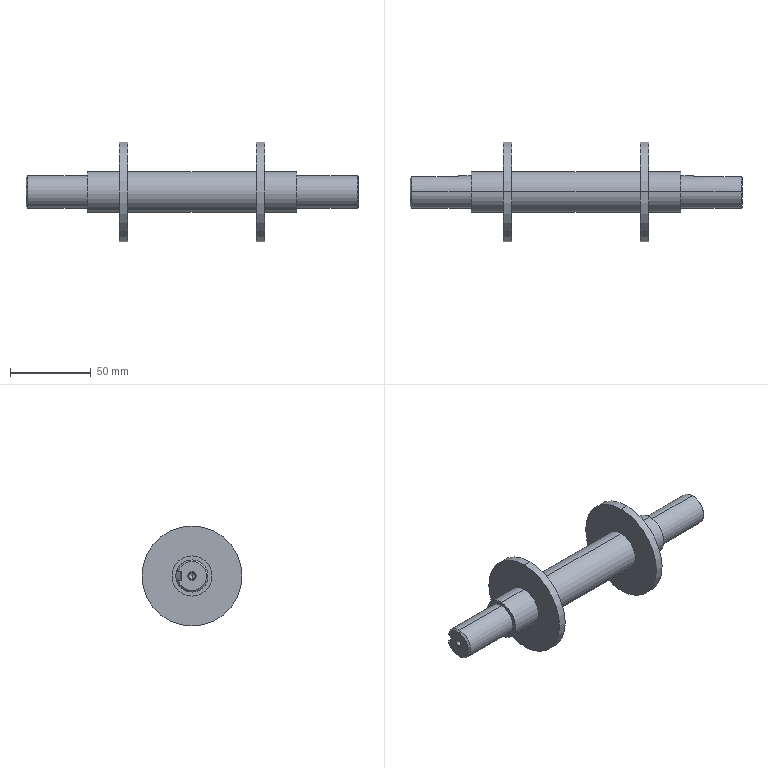Part | SolidWorks | features BaseBody 1 | 1 solid | 48 faces | box 206 x 62 x 62 mm | volume 111425 mm3 | cylinder 18 | cone 14 | plane 14 | spline 2 | commonest cylinder face diameters 25 x6 4.2 x4 20 x4 62 x4
STEP:
#1=CARTESIAN_POINT('',(102.5,0.,2.1));
#2=VERTEX_POINT('',#1);
#3=CARTESIAN_POINT('',(102.5,0.,-2.1));
#4=VERTEX_POINT('',#3);
#5=CARTESIAN_POINT('',(102.5,0.,0.));
#6=DIRECTION('',(1.,0.,0.));
#7=DIRECTION('',(0.,0.,-1.));
#8=AXIS2_PLACEMENT_3D('',#5,#6,#7);
#9=CIRCLE('',#8,2.1);
#10=EDGE_CURVE('',#2,#4,#9,.T.);
#11=ORIENTED_EDGE('',*,*,#10,.F.);
#12=CARTESIAN_POINT('',(103.,0.,2.6));
#13=VERTEX_POINT('',#12);
#14=CARTESIAN_POINT('',(102.5,0.,2.1));
#15=DIRECTION('',(0.7071,0.,0.7071));
#16=VECTOR('',#15,1000.);
#17=LINE('',#14,#16);
#18=EDGE_CURVE('',#2,#13,#17,.T.);
#19=ORIENTED_EDGE('',*,*,#18,.T.);
#20=CARTESIAN_POINT('',(103.,0.,-2.6));
#21=VERTEX_POINT('',#20);
#22=CARTESIAN_POINT('',(103.,0.,0.));
#23=DIRECTION('',(-1.,0.,0.));
#24=DIRECTION('',(0.,0.,-1.));
#25=AXIS2_PLACEMENT_3D('',#22,#23,#24);
#26=CIRCLE('',#25,2.6);
#27=EDGE_CURVE('',#21,#13,#26,.T.);
#28=ORIENTED_EDGE('',*,*,#27,.F.);
#29=CARTESIAN_POINT('',(102.5,0.,-2.1));
#30=DIRECTION('',(0.7071,0.,-0.7071));
#31=VECTOR('',#30,1000.);
#32=LINE('',#29,#31);
#33=EDGE_CURVE('',#4,#21,#32,.T.);
#34=ORIENTED_EDGE('',*,*,#33,.F.);
#35=EDGE_LOOP('',(#11,#19,#28,#34));
#36=FACE_OUTER_BOUND('',#35,.T.);
#37=CARTESIAN_POINT('',(102.5,0.,0.));
#38=DIRECTION('',(1.,0.,0.));
#39=DIRECTION('',(0.,0.,-1.));
#40=AXIS2_PLACEMENT_3D('',#37,#38,#39);
#41=CONICAL_SURFACE('',#40,2.1,0.7854);
#42=ADVANCED_FACE('',(#36),#41,.F.);
#43=CARTESIAN_POINT('',(-102.5,0.,-2.1));
#44=VERTEX_POINT('',#43);
#45=CARTESIAN_POINT('',(-102.5,0.,2.1));
#46=VERTEX_POINT('',#45);
#47=CARTESIAN_POINT('',(-102.5,0.,0.));
#48=DIRECTION('',(-1.,0.,0.));
#49=DIRECTION('',(0.,0.,1.));
#50=AXIS2_PLACEMENT_3D('',#47,#48,#49);
#51=CIRCLE('',#50,2.1);
#52=EDGE_CURVE('',#44,#46,#51,.T.);
#53=ORIENTED_EDGE('',*,*,#52,.F.);
#54=CARTESIAN_POINT('',(-103.,0.,-2.6));
#55=VERTEX_POINT('',#54);
#56=CARTESIAN_POINT('',(-102.5,0.,-2.1));
#57=DIRECTION('',(-0.7071,0.,-0.7071));
#58=VECTOR('',#57,1000.);
#59=LINE('',#56,#58);
#60=EDGE_CURVE('',#44,#55,#59,.T.);
#61=ORIENTED_EDGE('',*,*,#60,.T.);
#62=CARTESIAN_POINT('',(-103.,0.,2.6));
#63=VERTEX_POINT('',#62);
#64=CARTESIAN_POINT('',(-103.,0.,0.));
#65=DIRECTION('',(1.,0.,0.));
#66=DIRECTION('',(0.,0.,1.));
#67=AXIS2_PLACEMENT_3D('',#64,#65,#66);
#68=CIRCLE('',#67,2.6);
#69=EDGE_CURVE('',#63,#55,#68,.T.);
#70=ORIENTED_EDGE('',*,*,#69,.F.);
#71=CARTESIAN_POINT('',(-102.5,0.,2.1));
#72=DIRECTION('',(-0.7071,0.,0.7071));
#73=VECTOR('',#72,1000.);
#74=LINE('',#71,#73);
#75=EDGE_CURVE('',#46,#63,#74,.T.);
#76=ORIENTED_EDGE('',*,*,#75,.F.);
#77=EDGE_LOOP('',(#53,#61,#70,#76));
#78=FACE_OUTER_BOUND('',#77,.T.);
#79=CARTESIAN_POINT('',(-102.5,0.,0.));
#80=DIRECTION('',(-1.,0.,0.));
#81=DIRECTION('',(0.,0.,1.));
#82=AXIS2_PLACEMENT_3D('',#79,#80,#81);
#83=CONICAL_SURFACE('',#82,2.1,0.7854);
#84=ADVANCED_FACE('',(#78),#83,.F.);
#85=CARTESIAN_POINT('',(90.6,0.,2.1));
#86=VERTEX_POINT('',#85);
#87=CARTESIAN_POINT('',(90.6,0.,-2.1));
#88=VERTEX_POINT('',#87);
#89=CARTESIAN_POINT('',(90.6,0.,0.));
#90=DIRECTION('',(1.,0.,0.));
#91=DIRECTION('',(0.,0.,-1.));
#92=AXIS2_PLACEMENT_3D('',#89,#90,#91);
#93=CIRCLE('',#92,2.1);
#94=EDGE_CURVE('',#86,#88,#93,.T.);
#95=ORIENTED_EDGE('',*,*,#94,.F.);
#96=CARTESIAN_POINT('',(103.,0.,2.1));
#97=DIRECTION('',(1.,0.,0.));
#98=VECTOR('',#97,1000.);
#99=LINE('',#96,#98);
#100=EDGE_CURVE('',#86,#2,#99,.T.);
#101=ORIENTED_EDGE('',*,*,#100,.T.);
#102=ORIENTED_EDGE('',*,*,#10,.T.);
#103=CARTESIAN_POINT('',(103.,0.,-2.1));
#104=DIRECTION('',(1.,0.,0.));
#105=VECTOR('',#104,1000.);
#106=LINE('',#103,#105);
#107=EDGE_CURVE('',#88,#4,#106,.T.);
#108=ORIENTED_EDGE('',*,*,#107,.F.);
#109=EDGE_LOOP('',(#95,#101,#102,#108));
#110=FACE_OUTER_BOUND('',#109,.T.);
#111=CARTESIAN_POINT('',(103.,0.,0.));
#112=DIRECTION('',(1.,0.,0.));
#113=DIRECTION('',(0.,0.,-1.));
#114=AXIS2_PLACEMENT_3D('',#111,#112,#113);
#115=CYLINDRICAL_SURFACE('',#114,2.1);
#116=ADVANCED_FACE('',(#110),#115,.F.);
#117=CARTESIAN_POINT('',(89.338,0.,0.));
#118=VERTEX_POINT('',#117);
#119=CARTESIAN_POINT('',(90.6,0.,-2.1));
#120=DIRECTION('',(0.515,0.,-0.8572));
#121=VECTOR('',#120,1000.);
#122=LINE('',#119,#121);
#123=EDGE_CURVE('',#118,#88,#122,.T.);
#124=ORIENTED_EDGE('',*,*,#123,.F.);
#125=CARTESIAN_POINT('',(90.6,0.,2.1));
#126=DIRECTION('',(0.515,0.,0.8572));
#127=VECTOR('',#126,1000.);
#128=LINE('',#125,#127);
#129=EDGE_CURVE('',#118,#86,#128,.T.);
#130=ORIENTED_EDGE('',*,*,#129,.T.);
#131=ORIENTED_EDGE('',*,*,#94,.T.);
#132=EDGE_LOOP('',(#124,#130,#131));
#133=FACE_OUTER_BOUND('',#132,.T.);
#134=CARTESIAN_POINT('',(90.6,0.,0.));
#135=DIRECTION('',(1.,0.,0.));
#136=DIRECTION('',(0.,0.,-1.));
#137=AXIS2_PLACEMENT_3D('',#134,#135,#136);
#138=CONICAL_SURFACE('',#137,2.1,1.03);
#139=ADVANCED_FACE('',(#133),#138,.F.);
#140=CARTESIAN_POINT('',(-90.6,0.,-2.1));
#141=VERTEX_POINT('',#140);
#142=CARTESIAN_POINT('',(-90.6,0.,2.1));
#143=VERTEX_POINT('',#142);
#144=CARTESIAN_POINT('',(-90.6,0.,0.));
#145=DIRECTION('',(-1.,0.,0.));
#146=DIRECTION('',(0.,0.,1.));
#147=AXIS2_PLACEMENT_3D('',#144,#145,#146);
#148=CIRCLE('',#147,2.1);
#149=EDGE_CURVE('',#141,#143,#148,.T.);
#150=ORIENTED_EDGE('',*,*,#149,.F.);
#151=CARTESIAN_POINT('',(-103.,0.,-2.1));
#152=DIRECTION('',(-1.,0.,0.));
#153=VECTOR('',#152,1000.);
#154=LINE('',#151,#153);
#155=EDGE_CURVE('',#141,#44,#154,.T.);
#156=ORIENTED_EDGE('',*,*,#155,.T.);
#157=ORIENTED_EDGE('',*,*,#52,.T.);
#158=CARTESIAN_POINT('',(-103.,0.,2.1));
#159=DIRECTION('',(-1.,0.,0.));
#160=VECTOR('',#159,1000.);
#161=LINE('',#158,#160);
#162=EDGE_CURVE('',#143,#46,#161,.T.);
#163=ORIENTED_EDGE('',*,*,#162,.F.);
#164=EDGE_LOOP('',(#150,#156,#157,#163));
#165=FACE_OUTER_BOUND('',#164,.T.);
#166=CARTESIAN_POINT('',(-103.,0.,0.));
#167=DIRECTION('',(-1.,0.,0.));
#168=DIRECTION('',(0.,0.,1.));
#169=AXIS2_PLACEMENT_3D('',#166,#167,#168);
#170=CYLINDRICAL_SURFACE('',#169,2.1);
#171=ADVANCED_FACE('',(#165),#170,.F.);
#172=CARTESIAN_POINT('',(-89.338,0.,0.));
#173=VERTEX_POINT('',#172);
#174=CARTESIAN_POINT('',(-90.6,0.,2.1));
#175=DIRECTION('',(-0.515,0.,0.8572));
#176=VECTOR('',#175,1000.);
#177=LINE('',#174,#176);
#178=EDGE_CURVE('',#173,#143,#177,.T.);
#179=ORIENTED_EDGE('',*,*,#178,.F.);
#180=CARTESIAN_POINT('',(-90.6,0.,-2.1));
#181=DIRECTION('',(-0.515,0.,-0.8572));
#182=VECTOR('',#181,1000.);
#183=LINE('',#180,#182);
#184=EDGE_CURVE('',#173,#141,#183,.T.);
#185=ORIENTED_EDGE('',*,*,#184,.T.);
#186=ORIENTED_EDGE('',*,*,#149,.T.);
#187=EDGE_LOOP('',(#179,#185,#186));
#188=FACE_OUTER_BOUND('',#187,.T.);
#189=CARTESIAN_POINT('',(-90.6,0.,0.));
#190=DIRECTION('',(-1.,0.,0.));
#191=DIRECTION('',(0.,0.,1.));
#192=AXIS2_PLACEMENT_3D('',#189,#190,#191);
#193=CONICAL_SURFACE('',#192,2.1,1.03);
#194=ADVANCED_FACE('',(#188),#193,.F.);
#195=CARTESIAN_POINT('',(-103.,0.,9.));
#196=VERTEX_POINT('',#195);
#197=CARTESIAN_POINT('',(-103.,8.485,3.));
#198=VERTEX_POINT('',#197);
#199=CARTESIAN_POINT('',(-103.,0.,0.));
#200=DIRECTION('',(-1.,0.,0.));
#201=DIRECTION('',(0.,0.,1.));
#202=AXIS2_PLACEMENT_3D('',#199,#200,#201);
#203=CIRCLE('',#202,9.);
#204=EDGE_CURVE('',#196,#198,#203,.T.);
#205=ORIENTED_EDGE('',*,*,#204,.F.);
#206=CARTESIAN_POINT('',(-102.,0.,10.));
#207=VERTEX_POINT('',#206);
#208=CARTESIAN_POINT('',(-103.,0.,9.));
#209=DIRECTION('',(0.7071,0.,0.7071));
#210=VECTOR('',#209,1000.);
#211=LINE('',#208,#210);
#212=EDGE_CURVE('',#196,#207,#211,.T.);
#213=ORIENTED_EDGE('',*,*,#212,.T.);
#214=CARTESIAN_POINT('',(-102.,9.539,3.));
#215=VERTEX_POINT('',#214);
#216=CARTESIAN_POINT('',(-102.,0.,0.));
#217=DIRECTION('',(1.,0.,0.));
#218=DIRECTION('',(0.,0.,1.));
#219=AXIS2_PLACEMENT_3D('',#216,#217,#218);
#220=CIRCLE('',#219,10.);
#221=EDGE_CURVE('',#215,#207,#220,.T.);
#222=ORIENTED_EDGE('',*,*,#221,.F.);
#223=CARTESIAN_POINT('',(-103.,8.485,3.));
#224=CARTESIAN_POINT('',(-102.668,8.838,3.));
#225=CARTESIAN_POINT('',(-102.334,9.189,3.));
#226=CARTESIAN_POINT('',(-102.,9.539,3.));
#227=B_SPLINE_CURVE_WITH_KNOTS('',3,(#223,#224,#225,#226),.UNSPECIFIED.,.F.,.F.,(4,4),(0.006491,0.007944),.UNSPECIFIED.);
#228=EDGE_CURVE('',#198,#215,#227,.T.);
#229=ORIENTED_EDGE('',*,*,#228,.F.);
#230=EDGE_LOOP('',(#205,#213,#222,#229));
#231=FACE_OUTER_BOUND('',#230,.T.);
#232=CARTESIAN_POINT('',(-103.,0.,0.));
#233=DIRECTION('',(1.,0.,0.));
#234=DIRECTION('',(0.,0.,-1.));
#235=AXIS2_PLACEMENT_3D('',#232,#233,#234);
#236=CONICAL_SURFACE('',#235,9.,0.7854);
#237=ADVANCED_FACE('',(#231),#236,.T.);
#238=ORIENTED_EDGE('',*,*,#212,.F.);
#239=CARTESIAN_POINT('',(-103.,0.,-9.));
#240=VERTEX_POINT('',#239);
#241=CARTESIAN_POINT('',(-103.,0.,0.));
#242=DIRECTION('',(-1.,0.,0.));
#243=DIRECTION('',(0.,0.,1.));
#244=AXIS2_PLACEMENT_3D('',#241,#242,#243);
#245=CIRCLE('',#244,9.);
#246=EDGE_CURVE('',#240,#196,#245,.T.);
#247=ORIENTED_EDGE('',*,*,#246,.F.);
#248=CARTESIAN_POINT('',(-102.,0.,-10.));
#249=VERTEX_POINT('',#248);
#250=CARTESIAN_POINT('',(-103.,0.,-9.));
#251=DIRECTION('',(0.7071,0.,-0.7071));
#252=VECTOR('',#251,1000.);
#253=LINE('',#250,#252);
#254=EDGE_CURVE('',#240,#249,#253,.T.);
#255=ORIENTED_EDGE('',*,*,#254,.T.);
#256=CARTESIAN_POINT('',(-102.,0.,0.));
#257=DIRECTION('',(1.,0.,0.));
#258=DIRECTION('',(0.,0.,1.));
#259=AXIS2_PLACEMENT_3D('',#256,#257,#258);
#260=CIRCLE('',#259,10.);
#261=EDGE_CURVE('',#207,#249,#260,.T.);
#262=ORIENTED_EDGE('',*,*,#261,.F.);
#263=EDGE_LOOP('',(#238,#247,#255,#262));
#264=FACE_OUTER_BOUND('',#263,.T.);
#265=CARTESIAN_POINT('',(-103.,0.,0.));
#266=DIRECTION('',(1.,0.,0.));
#267=DIRECTION('',(0.,0.,-1.));
#268=AXIS2_PLACEMENT_3D('',#265,#266,#267);
#269=CONICAL_SURFACE('',#268,9.,0.7854);
#270=ADVANCED_FACE('',(#264),#269,.T.);
#271=ORIENTED_EDGE('',*,*,#221,.T.);
#272=CARTESIAN_POINT('',(-65.,0.,10.));
#273=VERTEX_POINT('',#272);
#274=CARTESIAN_POINT('',(-103.,0.,10.));
#275=DIRECTION('',(1.,0.,0.));
#276=VECTOR('',#275,1000.);
#277=LINE('',#274,#276);
#278=EDGE_CURVE('',#207,#273,#277,.T.);
#279=ORIENTED_EDGE('',*,*,#278,.T.);
#280=CARTESIAN_POINT('',(-65.,0.,-10.));
#281=VERTEX_POINT('',#280);
#282=CARTESIAN_POINT('',(-65.,0.,0.));
#283=DIRECTION('',(-1.,0.,0.));
#284=DIRECTION('',(0.,0.,1.));
#285=AXIS2_PLACEMENT_3D('',#282,#283,#284);
#286=CIRCLE('',#285,10.);
#287=EDGE_CURVE('',#273,#281,#286,.T.);
#288=ORIENTED_EDGE('',*,*,#287,.T.);
#289=CARTESIAN_POINT('',(-103.,0.,-10.));
#290=DIRECTION('',(1.,0.,0.));
#291=VECTOR('',#290,1000.);
#292=LINE('',#289,#291);
#293=EDGE_CURVE('',#249,#281,#292,.T.);
#294=ORIENTED_EDGE('',*,*,#293,.F.);
#295=CARTESIAN_POINT('',(-102.,9.539,-3.));
#296=VERTEX_POINT('',#295);
#297=CARTESIAN_POINT('',(-102.,0.,0.));
#298=DIRECTION('',(1.,0.,0.));
#299=DIRECTION('',(0.,0.,1.));
#300=AXIS2_PLACEMENT_3D('',#297,#298,#299);
#301=CIRCLE('',#300,10.);
#302=EDGE_CURVE('',#249,#296,#301,.T.);
#303=ORIENTED_EDGE('',*,*,#302,.T.);
#304=CARTESIAN_POINT('',(-73.,9.539,-3.));
#305=VERTEX_POINT('',#304);
#306=CARTESIAN_POINT('',(-103.,9.539,-3.));
#307=DIRECTION('',(1.,0.,0.));
#308=VECTOR('',#307,1000.);
#309=LINE('',#306,#308);
#310=EDGE_CURVE('',#296,#305,#309,.T.);
#311=ORIENTED_EDGE('',*,*,#310,.T.);
#312=CARTESIAN_POINT('',(-73.,9.539,3.));
#313=VERTEX_POINT('',#312);
#314=CARTESIAN_POINT('',(-73.,9.539,-3.));
#315=CARTESIAN_POINT('',(-73.,9.692,-2.514));
#316=CARTESIAN_POINT('',(-73.,9.807,-2.019));
#317=CARTESIAN_POINT('',(-73.,9.962,-1.011));
#318=CARTESIAN_POINT('',(-73.,10.,-0.5036));
#319=CARTESIAN_POINT('',(-73.,10.,0.5143));
#320=CARTESIAN_POINT('',(-73.,9.96,1.022));
#321=CARTESIAN_POINT('',(-73.,9.807,2.021));
#322=CARTESIAN_POINT('',(-73.,9.692,2.514));
#323=CARTESIAN_POINT('',(-73.,9.539,3.));
#324=B_SPLINE_CURVE_WITH_KNOTS('',3,(#314,#315,#316,#317,#318,#319,#320,#321,#322,#323),.UNSPECIFIED.,.F.,.F.,(4,2,2,2,4),(0.,0.001525,0.003049,0.004574,0.006098),.UNSPECIFIED.);
#325=EDGE_CURVE('',#305,#313,#324,.T.);
#326=ORIENTED_EDGE('',*,*,#325,.T.);
#327=CARTESIAN_POINT('',(-103.,9.539,3.));
#328=DIRECTION('',(-1.,0.,0.));
#329=VECTOR('',#328,1000.);
#330=LINE('',#327,#329);
#331=EDGE_CURVE('',#313,#215,#330,.T.);
#332=ORIENTED_EDGE('',*,*,#331,.T.);
#333=EDGE_LOOP('',(#271,#279,#288,#294,#303,#311,#326,#332));
#334=FACE_OUTER_BOUND('',#333,.T.);
#335=CARTESIAN_POINT('',(-103.,0.,0.));
#336=DIRECTION('',(1.,0.,0.));
#337=DIRECTION('',(0.,0.,-1.));
#338=AXIS2_PLACEMENT_3D('',#335,#336,#337);
#339=CYLINDRICAL_SURFACE('',#338,10.);
#340=ADVANCED_FACE('',(#334),#339,.T.);
#341=CARTESIAN_POINT('',(65.,0.,12.5));
#342=VERTEX_POINT('',#341);
#343=CARTESIAN_POINT('',(65.,0.,-12.5));
#344=VERTEX_POINT('',#343);
#345=CARTESIAN_POINT('',(65.,0.,0.));
#346=DIRECTION('',(-1.,0.,0.));
#347=DIRECTION('',(0.,0.,1.));
#348=AXIS2_PLACEMENT_3D('',#345,#346,#347);
#349=CIRCLE('',#348,12.5);
#350=EDGE_CURVE('',#342,#344,#349,.T.);
#351=ORIENTED_EDGE('',*,*,#350,.T.);
#352=CARTESIAN_POINT('',(45.,0.,-12.5));
#353=VERTEX_POINT('',#352);
#354=CARTESIAN_POINT('',(-45.,0.,-12.5));
#355=DIRECTION('',(-1.,0.,0.));
#356=VECTOR('',#355,1000.);
#357=LINE('',#354,#356);
#358=EDGE_CURVE('',#344,#353,#357,.T.);
#359=ORIENTED_EDGE('',*,*,#358,.T.);
#360=CARTESIAN_POINT('',(45.,0.,12.5));
#361=VERTEX_POINT('',#360);
#362=CARTESIAN_POINT('',(45.,0.,0.));
#363=DIRECTION('',(-1.,0.,0.));
#364=DIRECTION('',(0.,0.,1.));
#365=AXIS2_PLACEMENT_3D('',#362,#363,#364);
#366=CIRCLE('',#365,12.5);
#367=EDGE_CURVE('',#361,#353,#366,.T.);
#368=ORIENTED_EDGE('',*,*,#367,.F.);
#369=CARTESIAN_POINT('',(-45.,0.,12.5));
#370=DIRECTION('',(-1.,0.,0.));
#371=VECTOR('',#370,1000.);
#372=LINE('',#369,#371);
#373=EDGE_CURVE('',#342,#361,#372,.T.);
#374=ORIENTED_EDGE('',*,*,#373,.F.);
#375=EDGE_LOOP('',(#351,#359,#368,#374));
#376=FACE_OUTER_BOUND('',#375,.T.);
#377=CARTESIAN_POINT('',(-45.,0.,0.));
#378=DIRECTION('',(-1.,0.,0.));
#379=DIRECTION('',(0.,0.,1.));
#380=AXIS2_PLACEMENT_3D('',#377,#378,#379);
#381=CYLINDRICAL_SURFACE('',#380,12.5);
#382=ADVANCED_FACE('',(#376),#381,.T.);
#383=CARTESIAN_POINT('',(45.,0.,31.));
#384=VERTEX_POINT('',#383);
#385=CARTESIAN_POINT('',(45.,0.,-31.));
#386=VERTEX_POINT('',#385);
#387=CARTESIAN_POINT('',(45.,0.,0.));
#388=DIRECTION('',(-1.,0.,0.));
#389=DIRECTION('',(0.,0.,1.));
#390=AXIS2_PLACEMENT_3D('',#387,#388,#389);
#391=CIRCLE('',#390,31.);
#392=EDGE_CURVE('',#384,#386,#391,.T.);
#393=ORIENTED_EDGE('',*,*,#392,.T.);
#394=CARTESIAN_POINT('',(40.,0.,-31.));
#395=VERTEX_POINT('',#394);
#396=CARTESIAN_POINT('',(-45.,0.,-31.));
#397=DIRECTION('',(-1.,0.,0.));
#398=VECTOR('',#397,1000.);
#399=LINE('',#396,#398);
#400=EDGE_CURVE('',#386,#395,#399,.T.);
#401=ORIENTED_EDGE('',*,*,#400,.T.);
#402=CARTESIAN_POINT('',(40.,0.,31.));
#403=VERTEX_POINT('',#402);
#404=CARTESIAN_POINT('',(40.,0.,0.));
#405=DIRECTION('',(1.,0.,0.));
#406=DIRECTION('',(0.,0.,-1.));
#407=AXIS2_PLACEMENT_3D('',#404,#405,#406);
#408=CIRCLE('',#407,31.);
#409=EDGE_CURVE('',#395,#403,#408,.T.);
#410=ORIENTED_EDGE('',*,*,#409,.T.);
#411=CARTESIAN_POINT('',(-45.,0.,31.));
#412=DIRECTION('',(-1.,0.,0.));
#413=VECTOR('',#412,1000.);
#414=LINE('',#411,#413);
#415=EDGE_CURVE('',#384,#403,#414,.T.);
#416=ORIENTED_EDGE('',*,*,#415,.F.);
#417=EDGE_LOOP('',(#393,#401,#410,#416));
#418=FACE_OUTER_BOUND('',#417,.T.);
#419=CARTESIAN_POINT('',(-45.,0.,0.));
#420=DIRECTION('',(-1.,0.,0.));
#421=DIRECTION('',(0.,0.,1.));
#422=AXIS2_PLACEMENT_3D('',#419,#420,#421);
#423=CYLINDRICAL_SURFACE('',#422,31.);
#424=ADVANCED_FACE('',(#418),#423,.T.);
#425=CARTESIAN_POINT('',(-45.,0.,12.5));
#426=VERTEX_POINT('',#425);
#427=CARTESIAN_POINT('',(-45.,0.,-12.5));
#428=VERTEX_POINT('',#427);
#429=CARTESIAN_POINT('',(-45.,0.,0.));
#430=DIRECTION('',(-1.,0.,0.));
#431=DIRECTION('',(0.,0.,-1.));
#432=AXIS2_PLACEMENT_3D('',#429,#430,#431);
#433=CIRCLE('',#432,12.5);
#434=EDGE_CURVE('',#426,#428,#433,.T.);
#435=ORIENTED_EDGE('',*,*,#434,.T.);
#436=CARTESIAN_POINT('',(-65.,0.,-12.5));
#437=VERTEX_POINT('',#436);
#438=CARTESIAN_POINT('',(-45.,0.,-12.5));
#439=DIRECTION('',(-1.,0.,0.));
#440=VECTOR('',#439,1000.);
#441=LINE('',#438,#440);
#442=EDGE_CURVE('',#428,#437,#441,.T.);
#443=ORIENTED_EDGE('',*,*,#442,.T.);
#444=CARTESIAN_POINT('',(-65.,0.,12.5));
#445=VERTEX_POINT('',#444);
#446=CARTESIAN_POINT('',(-65.,0.,0.));
#447=DIRECTION('',(-1.,0.,0.));
#448=DIRECTION('',(0.,0.,1.));
#449=AXIS2_PLACEMENT_3D('',#446,#447,#448);
#450=CIRCLE('',#449,12.5);
#451=EDGE_CURVE('',#445,#437,#450,.T.);
#452=ORIENTED_EDGE('',*,*,#451,.F.);
#453=CARTESIAN_POINT('',(-45.,0.,12.5));
#454=DIRECTION('',(-1.,0.,0.));
#455=VECTOR('',#454,1000.);
#456=LINE('',#453,#455);
#457=EDGE_CURVE('',#426,#445,#456,.T.);
#458=ORIENTED_EDGE('',*,*,#457,.F.);
#459=EDGE_LOOP('',(#435,#443,#452,#458));
#460=FACE_OUTER_BOUND('',#459,.T.);
#461=CARTESIAN_POINT('',(-45.,0.,0.));
#462=DIRECTION('',(-1.,0.,0.));
#463=DIRECTION('',(0.,0.,1.));
#464=AXIS2_PLACEMENT_3D('',#461,#462,#463);
#465=CYLINDRICAL_SURFACE('',#464,12.5);
#466=ADVANCED_FACE('',(#460),#465,.T.);
#467=CARTESIAN_POINT('',(-40.,0.,-31.));
#468=VERTEX_POINT('',#467);
#469=CARTESIAN_POINT('',(-40.,0.,31.));
#470=VERTEX_POINT('',#469);
#471=CARTESIAN_POINT('',(-40.,0.,0.));
#472=DIRECTION('',(1.,0.,0.));
#473=DIRECTION('',(0.,0.,-1.));
#474=AXIS2_PLACEMENT_3D('',#471,#472,#473);
#475=CIRCLE('',#474,31.);
#476=EDGE_CURVE('',#468,#470,#475,.T.);
#477=ORIENTED_EDGE('',*,*,#476,.F.);
#478=CARTESIAN_POINT('',(-45.,0.,-31.));
#479=VERTEX_POINT('',#478);
#480=CARTESIAN_POINT('',(-45.,0.,-31.));
#481=DIRECTION('',(-1.,0.,0.));
#482=VECTOR('',#481,1000.);
#483=LINE('',#480,#482);
#484=EDGE_CURVE('',#468,#479,#483,.T.);
#485=ORIENTED_EDGE('',*,*,#484,.T.);
#486=CARTESIAN_POINT('',(-45.,0.,31.));
#487=VERTEX_POINT('',#486);
#488=CARTESIAN_POINT('',(-45.,0.,0.));
#489=DIRECTION('',(-1.,0.,0.));
#490=DIRECTION('',(0.,0.,1.));
#491=AXIS2_PLACEMENT_3D('',#488,#489,#490);
#492=CIRCLE('',#491,31.);
#493=EDGE_CURVE('',#487,#479,#492,.T.);
#494=ORIENTED_EDGE('',*,*,#493,.F.);
#495=CARTESIAN_POINT('',(-45.,0.,31.));
#496=DIRECTION('',(-1.,0.,0.));
#497=VECTOR('',#496,1000.);
#498=LINE('',#495,#497);
#499=EDGE_CURVE('',#470,#487,#498,.T.);
#500=ORIENTED_EDGE('',*,*,#499,.F.);
#501=EDGE_LOOP('',(#477,#485,#494,#500));
#502=FACE_OUTER_BOUND('',#501,.T.);
#503=CARTESIAN_POINT('',(-45.,0.,0.));
#504=DIRECTION('',(-1.,0.,0.));
#505=DIRECTION('',(0.,0.,1.));
#506=AXIS2_PLACEMENT_3D('',#503,#504,#505);
#507=CYLINDRICAL_SURFACE('',#506,31.);
#508=ADVANCED_FACE('',(#502),#507,.T.);
#509=CARTESIAN_POINT('',(40.,0.,-12.5));
#510=VERTEX_POINT('',#509);
#511=CARTESIAN_POINT('',(40.,0.,12.5));
#512=VERTEX_POINT('',#511);
#513=CARTESIAN_POINT('',(40.,0.,0.));
#514=DIRECTION('',(1.,0.,0.));
#515=DIRECTION('',(0.,0.,-1.));
#516=AXIS2_PLACEMENT_3D('',#513,#514,#515);
#517=CIRCLE('',#516,12.5);
#518=EDGE_CURVE('',#510,#512,#517,.T.);
#519=ORIENTED_EDGE('',*,*,#518,.F.);
#520=CARTESIAN_POINT('',(-40.,0.,-12.5));
#521=VERTEX_POINT('',#520);
#522=CARTESIAN_POINT('',(-45.,0.,-12.5));
#523=DIRECTION('',(-1.,0.,0.));
#524=VECTOR('',#523,1000.);
#525=LINE('',#522,#524);
#526=EDGE_CURVE('',#510,#521,#525,.T.);
#527=ORIENTED_EDGE('',*,*,#526,.T.);
#528=CARTESIAN_POINT('',(-40.,0.,12.5));
#529=VERTEX_POINT('',#528);
#530=CARTESIAN_POINT('',(-40.,0.,0.));
#531=DIRECTION('',(1.,0.,0.));
#532=DIRECTION('',(0.,0.,-1.));
#533=AXIS2_PLACEMENT_3D('',#530,#531,#532);
#534=CIRCLE('',#533,12.5);
#535=EDGE_CURVE('',#521,#529,#534,.T.);
#536=ORIENTED_EDGE('',*,*,#535,.T.);
#537=CARTESIAN_POINT('',(-45.,0.,12.5));
#538=DIRECTION('',(-1.,0.,0.));
#539=VECTOR('',#538,1000.);
#540=LINE('',#537,#539);
#541=EDGE_CURVE('',#512,#529,#540,.T.);
#542=ORIENTED_EDGE('',*,*,#541,.F.);
#543=EDGE_LOOP('',(#519,#527,#536,#542));
#544=FACE_OUTER_BOUND('',#543,.T.);
#545=CARTESIAN_POINT('',(-45.,0.,0.));
#546=DIRECTION('',(-1.,0.,0.));
#547=DIRECTION('',(0.,0.,1.));
#548=AXIS2_PLACEMENT_3D('',#545,#546,#547);
#549=CYLINDRICAL_SURFACE('',#548,12.5);
#550=ADVANCED_FACE('',(#544),#549,.T.);
#551=CARTESIAN_POINT('',(103.,0.,-9.5));
#552=VERTEX_POINT('',#551);
#553=CARTESIAN_POINT('',(103.,9.014,-3.));
#554=VERTEX_POINT('',#553);
#555=CARTESIAN_POINT('',(103.,0.,0.));
#556=DIRECTION('',(1.,0.,0.));
#557=DIRECTION('',(0.,0.,-1.));
#558=AXIS2_PLACEMENT_3D('',#555,#556,#557);
#559=CIRCLE('',#558,9.5);
#560=EDGE_CURVE('',#552,#554,#559,.T.);
#561=ORIENTED_EDGE('',*,*,#560,.F.);
#562=CARTESIAN_POINT('',(102.5,0.,-10.));
#563=VERTEX_POINT('',#562);
#564=CARTESIAN_POINT('',(103.,0.,-9.5));
#565=DIRECTION('',(-0.7071,0.,-0.7071));
#566=VECTOR('',#565,1000.);
#567=LINE('',#564,#566);
#568=EDGE_CURVE('',#552,#563,#567,.T.);
#569=ORIENTED_EDGE('',*,*,#568,.T.);
#570=CARTESIAN_POINT('',(102.5,9.539,-3.));
#571=VERTEX_POINT('',#570);
#572=CARTESIAN_POINT('',(102.5,0.,0.));
#573=DIRECTION('',(-1.,0.,0.));
#574=DIRECTION('',(0.,0.,-1.));
#575=AXIS2_PLACEMENT_3D('',#572,#573,#574);
#576=CIRCLE('',#575,10.);
#577=EDGE_CURVE('',#571,#563,#576,.T.);
#578=ORIENTED_EDGE('',*,*,#577,.F.);
#579=CARTESIAN_POINT('',(102.5,9.539,-3.));
#580=CARTESIAN_POINT('',(102.667,9.364,-3.));
#581=CARTESIAN_POINT('',(102.834,9.189,-3.));
#582=CARTESIAN_POINT('',(103.,9.014,-3.));
#583=B_SPLINE_CURVE_WITH_KNOTS('',3,(#579,#580,#581,#582),.UNSPECIFIED.,.F.,.F.,(4,4),(0.005686,0.006411),.UNSPECIFIED.);
#584=EDGE_CURVE('',#571,#554,#583,.T.);
#585=ORIENTED_EDGE('',*,*,#584,.T.);
#586=EDGE_LOOP('',(#561,#569,#578,#585));
#587=FACE_OUTER_BOUND('',#586,.T.);
#588=CARTESIAN_POINT('',(103.,0.,0.));
#589=DIRECTION('',(-1.,0.,0.));
#590=DIRECTION('',(0.,0.,1.));
#591=AXIS2_PLACEMENT_3D('',#588,#589,#590);
#592=CONICAL_SURFACE('',#591,9.5,0.7854);
#593=ADVANCED_FACE('',(#587),#592,.T.);
#594=ORIENTED_EDGE('',*,*,#568,.F.);
#595=CARTESIAN_POINT('',(103.,0.,9.5));
#596=VERTEX_POINT('',#595);
#597=CARTESIAN_POINT('',(103.,0.,0.));
#598=DIRECTION('',(1.,0.,0.));
#599=DIRECTION('',(0.,0.,-1.));
#600=AXIS2_PLACEMENT_3D('',#597,#598,#599);
#601=CIRCLE('',#600,9.5);
#602=EDGE_CURVE('',#596,#552,#601,.T.);
#603=ORIENTED_EDGE('',*,*,#602,.F.);
#604=CARTESIAN_POINT('',(102.5,0.,10.));
#605=VERTEX_POINT('',#604);
#606=CARTESIAN_POINT('',(103.,0.,9.5));
#607=DIRECTION('',(-0.7071,0.,0.7071));
#608=VECTOR('',#607,1000.);
#609=LINE('',#606,#608);
#610=EDGE_CURVE('',#596,#605,#609,.T.);
#611=ORIENTED_EDGE('',*,*,#610,.T.);
#612=CARTESIAN_POINT('',(102.5,0.,0.));
#613=DIRECTION('',(-1.,0.,0.));
#614=DIRECTION('',(0.,0.,-1.));
#615=AXIS2_PLACEMENT_3D('',#612,#613,#614);
#616=CIRCLE('',#615,10.);
#617=EDGE_CURVE('',#563,#605,#616,.T.);
#618=ORIENTED_EDGE('',*,*,#617,.F.);
#619=EDGE_LOOP('',(#594,#603,#611,#618));
#620=FACE_OUTER_BOUND('',#619,.T.);
#621=CARTESIAN_POINT('',(103.,0.,0.));
#622=DIRECTION('',(-1.,0.,0.));
#623=DIRECTION('',(0.,0.,1.));
#624=AXIS2_PLACEMENT_3D('',#621,#622,#623);
#625=CONICAL_SURFACE('',#624,9.5,0.7854);
#626=ADVANCED_FACE('',(#620),#625,.T.);
#627=ORIENTED_EDGE('',*,*,#577,.T.);
#628=CARTESIAN_POINT('',(65.,0.,-10.));
#629=VERTEX_POINT('',#628);
#630=CARTESIAN_POINT('',(103.,0.,-10.));
#631=DIRECTION('',(-1.,0.,0.));
#632=VECTOR('',#631,1000.);
#633=LINE('',#630,#632);
#634=EDGE_CURVE('',#563,#629,#633,.T.);
#635=ORIENTED_EDGE('',*,*,#634,.T.);
#636=CARTESIAN_POINT('',(65.,0.,10.));
#637=VERTEX_POINT('',#636);
#638=CARTESIAN_POINT('',(65.,0.,0.));
#639=DIRECTION('',(1.,0.,0.));
#640=DIRECTION('',(0.,0.,-1.));
#641=AXIS2_PLACEMENT_3D('',#638,#639,#640);
#642=CIRCLE('',#641,10.);
#643=EDGE_CURVE('',#629,#637,#642,.T.);
#644=ORIENTED_EDGE('',*,*,#643,.T.);
#645=CARTESIAN_POINT('',(103.,0.,10.));
#646=DIRECTION('',(-1.,0.,0.));
#647=VECTOR('',#646,1000.);
#648=LINE('',#645,#647);
#649=EDGE_CURVE('',#605,#637,#648,.T.);
#650=ORIENTED_EDGE('',*,*,#649,.F.);
#651=CARTESIAN_POINT('',(102.5,9.539,3.));
#652=VERTEX_POINT('',#651);
#653=CARTESIAN_POINT('',(102.5,0.,0.));
#654=DIRECTION('',(-1.,0.,0.));
#655=DIRECTION('',(0.,0.,-1.));
#656=AXIS2_PLACEMENT_3D('',#653,#654,#655);
#657=CIRCLE('',#656,10.);
#658=EDGE_CURVE('',#605,#652,#657,.T.);
#659=ORIENTED_EDGE('',*,*,#658,.T.);
#660=CARTESIAN_POINT('',(73.,9.539,3.));
#661=VERTEX_POINT('',#660);
#662=CARTESIAN_POINT('',(103.,9.539,3.));
#663=DIRECTION('',(1.,0.,0.));
#664=VECTOR('',#663,1000.);
#665=LINE('',#662,#664);
#666=EDGE_CURVE('',#661,#652,#665,.T.);
#667=ORIENTED_EDGE('',*,*,#666,.F.);
#668=CARTESIAN_POINT('',(73.,9.539,-3.));
#669=VERTEX_POINT('',#668);
#670=CARTESIAN_POINT('',(73.,9.539,3.));
#671=CARTESIAN_POINT('',(73.,9.692,2.514));
#672=CARTESIAN_POINT('',(73.,9.807,2.019));
#673=CARTESIAN_POINT('',(73.,9.962,1.011));
#674=CARTESIAN_POINT('',(73.,10.,0.5036));
#675=CARTESIAN_POINT('',(73.,10.,-0.5143));
#676=CARTESIAN_POINT('',(73.,9.96,-1.022));
#677=CARTESIAN_POINT('',(73.,9.807,-2.021));
#678=CARTESIAN_POINT('',(73.,9.692,-2.514));
#679=CARTESIAN_POINT('',(73.,9.539,-3.));
#680=B_SPLINE_CURVE_WITH_KNOTS('',3,(#670,#671,#672,#673,#674,#675,#676,#677,#678,#679),.UNSPECIFIED.,.F.,.F.,(4,2,2,2,4),(0.,0.001525,0.003049,0.004574,0.006098),.UNSPECIFIED.);
#681=EDGE_CURVE('',#661,#669,#680,.T.);
#682=ORIENTED_EDGE('',*,*,#681,.T.);
#683=CARTESIAN_POINT('',(103.,9.539,-3.));
#684=DIRECTION('',(-1.,0.,0.));
#685=VECTOR('',#684,1000.);
#686=LINE('',#683,#685);
#687=EDGE_CURVE('',#571,#669,#686,.T.);
#688=ORIENTED_EDGE('',*,*,#687,.F.);
#689=EDGE_LOOP('',(#627,#635,#644,#650,#659,#667,#682,#688));
#690=FACE_OUTER_BOUND('',#689,.T.);
#691=CARTESIAN_POINT('',(103.,0.,0.));
#692=DIRECTION('',(-1.,0.,0.));
#693=DIRECTION('',(0.,0.,1.));
#694=AXIS2_PLACEMENT_3D('',#691,#692,#693);
#695=CYLINDRICAL_SURFACE('',#694,10.);
#696=ADVANCED_FACE('',(#690),#695,.T.);
#697=CARTESIAN_POINT('',(77.631,6.5,-3.));
#698=VERTEX_POINT('',#697);
#699=CARTESIAN_POINT('',(73.,9.539,-3.));
#700=CARTESIAN_POINT('',(73.195,9.087,-3.));
#701=CARTESIAN_POINT('',(73.451,8.673,-3.));
#702=CARTESIAN_POINT('',(73.923,8.111,-3.));
#703=CARTESIAN_POINT('',(74.096,7.934,-3.));
#704=CARTESIAN_POINT('',(74.46,7.611,-3.));
#705=CARTESIAN_POINT('',(74.653,7.463,-3.));
#706=CARTESIAN_POINT('',(75.061,7.195,-3.));
#707=CARTESIAN_POINT('',(75.277,7.075,-3.));
#708=CARTESIAN_POINT('',(75.72,6.869,-3.));
#709=CARTESIAN_POINT('',(75.948,6.782,-3.));
#710=CARTESIAN_POINT('',(76.646,6.573,-3.));
#711=CARTESIAN_POINT('',(77.138,6.5,-3.));
#712=CARTESIAN_POINT('',(77.631,6.5,-3.));
#713=B_SPLINE_CURVE_WITH_KNOTS('',3,(#699,#700,#701,#702,#703,#704,#705,#706,#707,#708,#709,#710,#711,#712),.UNSPECIFIED.,.F.,.F.,(4,2,2,2,2,2,4),(0.,0.001458,0.002187,0.002915,0.003644,0.004373,0.005831),.UNSPECIFIED.);
#714=EDGE_CURVE('',#669,#698,#713,.T.);
#715=ORIENTED_EDGE('',*,*,#714,.F.);
#716=ORIENTED_EDGE('',*,*,#681,.F.);
#717=CARTESIAN_POINT('',(77.631,6.5,3.));
#718=VERTEX_POINT('',#717);
#719=CARTESIAN_POINT('',(77.631,6.5,3.));
#720=CARTESIAN_POINT('',(77.138,6.5,3.));
#721=CARTESIAN_POINT('',(76.657,6.571,3.));
#722=CARTESIAN_POINT('',(75.954,6.78,3.));
#723=CARTESIAN_POINT('',(75.722,6.868,3.));
#724=CARTESIAN_POINT('',(75.28,7.073,3.));
#725=CARTESIAN_POINT('',(75.068,7.191,3.));
#726=CARTESIAN_POINT('',(74.66,7.458,3.));
#727=CARTESIAN_POINT('',(74.463,7.608,3.));
#728=CARTESIAN_POINT('',(74.097,7.933,3.));
#729=CARTESIAN_POINT('',(73.927,8.107,3.));
#730=CARTESIAN_POINT('',(73.457,8.664,3.));
#731=CARTESIAN_POINT('',(73.195,9.087,3.));
#732=CARTESIAN_POINT('',(73.,9.539,3.));
#733=B_SPLINE_CURVE_WITH_KNOTS('',3,(#719,#720,#721,#722,#723,#724,#725,#726,#727,#728,#729,#730,#731,#732),.UNSPECIFIED.,.F.,.F.,(4,2,2,2,2,2,4),(0.,0.001458,0.002187,0.002916,0.003645,0.004373,0.005831),.UNSPECIFIED.);
#734=EDGE_CURVE('',#718,#661,#733,.T.);
#735=ORIENTED_EDGE('',*,*,#734,.F.);
#736=CARTESIAN_POINT('',(77.631,6.5,-3.));
#737=CARTESIAN_POINT('',(77.734,6.5,-2.002));
#738=CARTESIAN_POINT('',(77.77,6.5,-0.9991));
#739=CARTESIAN_POINT('',(77.77,6.5,1.002));
#740=CARTESIAN_POINT('',(77.734,6.5,2.002));
#741=CARTESIAN_POINT('',(77.631,6.5,3.));
#742=B_SPLINE_CURVE_WITH_KNOTS('',3,(#736,#737,#738,#739,#740,#741),.UNSPECIFIED.,.F.,.F.,(4,2,4),(0.,0.003008,0.006016),.UNSPECIFIED.);
#743=EDGE_CURVE('',#698,#718,#742,.T.);
#744=ORIENTED_EDGE('',*,*,#743,.F.);
#745=EDGE_LOOP('',(#715,#716,#735,#744));
#746=FACE_OUTER_BOUND('',#745,.T.);
#747=CARTESIAN_POINT('',(73.,9.529,3.032));
#748=CARTESIAN_POINT('',(74.287,6.5,3.21));
#749=CARTESIAN_POINT('',(77.552,6.5,3.66));
#750=CARTESIAN_POINT('',(73.,9.674,2.577));
#751=CARTESIAN_POINT('',(74.242,6.5,2.697));
#752=CARTESIAN_POINT('',(77.636,6.5,3.054));
#753=CARTESIAN_POINT('',(73.,9.793,2.088));
#754=CARTESIAN_POINT('',(74.194,6.5,2.175));
#755=CARTESIAN_POINT('',(77.688,6.5,2.447));
#756=CARTESIAN_POINT('',(73.,9.956,1.069));
#757=CARTESIAN_POINT('',(74.122,6.5,1.102));
#758=CARTESIAN_POINT('',(77.755,6.5,1.229));
#759=CARTESIAN_POINT('',(73.,10.,0.5385));
#760=CARTESIAN_POINT('',(74.101,6.5,0.5571));
#761=CARTESIAN_POINT('',(77.77,6.5,0.6192));
#762=CARTESIAN_POINT('',(73.,10.,-0.5242));
#763=CARTESIAN_POINT('',(74.101,6.5,-0.5423));
#764=CARTESIAN_POINT('',(77.77,6.5,-0.6028));
#765=CARTESIAN_POINT('',(73.,9.958,-1.056));
#766=CARTESIAN_POINT('',(74.122,6.5,-1.089));
#767=CARTESIAN_POINT('',(77.755,6.5,-1.215));
#768=CARTESIAN_POINT('',(73.,9.794,-2.084));
#769=CARTESIAN_POINT('',(74.193,6.5,-2.17));
#770=CARTESIAN_POINT('',(77.688,6.5,-2.441));
#771=CARTESIAN_POINT('',(73.,9.674,-2.576));
#772=CARTESIAN_POINT('',(74.242,6.5,-2.696));
#773=CARTESIAN_POINT('',(77.636,6.5,-3.052));
#774=CARTESIAN_POINT('',(73.,9.529,-3.033));
#775=CARTESIAN_POINT('',(74.287,6.5,-3.21));
#776=CARTESIAN_POINT('',(77.552,6.5,-3.66));
#777=(BOUNDED_SURFACE()B_SPLINE_SURFACE(3,2,((#747,#748,#749),(#750,#751,#752),(#753,#754,#755),(#756,#757,#758),(#759,#760,#761),(#762,#763,#764),(#765,#766,#767),(#768,#769,#770),(#771,#772,#773),(#774,#775,#776)),.UNSPECIFIED.,.F.,.F.,.T.)B_SPLINE_SURFACE_WITH_KNOTS((4,2,2,2,4),(3,3),(0.008171,0.01002,0.01187,0.01371,0.01556),(0.,1.),.UNSPECIFIED.)GEOMETRIC_REPRESENTATION_ITEM()RATIONAL_B_SPLINE_SURFACE(((1.,0.8349,1.),(1.,0.8262,1.),(1.,0.819,1.),(1.,0.809,1.),(1.,0.8062,1.),(1.,0.8062,1.),(1.,0.8089,1.),(1.,0.8189,1.),(1.,0.8262,1.),(1.,0.8349,1.)))REPRESENTATION_ITEM('')SURFACE());
#778=ADVANCED_FACE('',(#746),#777,.F.);
#779=CARTESIAN_POINT('',(103.,6.5,-3.));
#780=VERTEX_POINT('',#779);
#781=CARTESIAN_POINT('',(73.,6.5,-3.));
#782=DIRECTION('',(1.,0.,0.));
#783=VECTOR('',#782,1000.);
#784=LINE('',#781,#783);
#785=EDGE_CURVE('',#698,#780,#784,.T.);
#786=ORIENTED_EDGE('',*,*,#785,.F.);
#787=ORIENTED_EDGE('',*,*,#743,.T.);
#788=CARTESIAN_POINT('',(103.,6.5,3.));
#789=VERTEX_POINT('',#788);
#790=CARTESIAN_POINT('',(73.,6.5,3.));
#791=DIRECTION('',(1.,0.,0.));
#792=VECTOR('',#791,1000.);
#793=LINE('',#790,#792);
#794=EDGE_CURVE('',#718,#789,#793,.T.);
#795=ORIENTED_EDGE('',*,*,#794,.T.);
#796=CARTESIAN_POINT('',(103.,6.5,-3.));
#797=DIRECTION('',(0.,0.,1.));
#798=VECTOR('',#797,1000.);
#799=LINE('',#796,#798);
#800=EDGE_CURVE('',#780,#789,#799,.T.);
#801=ORIENTED_EDGE('',*,*,#800,.F.);
#802=EDGE_LOOP('',(#786,#787,#795,#801));
#803=FACE_OUTER_BOUND('',#802,.T.);
#804=CARTESIAN_POINT('',(73.,6.5,-3.));
#805=DIRECTION('',(0.,1.,0.));
#806=DIRECTION('',(0.,0.,-1.));
#807=AXIS2_PLACEMENT_3D('',#804,#805,#806);
#808=PLANE('',#807);
#809=ADVANCED_FACE('',(#803),#808,.T.);
#810=ORIENTED_EDGE('',*,*,#794,.F.);
#811=ORIENTED_EDGE('',*,*,#734,.T.);
#812=ORIENTED_EDGE('',*,*,#666,.T.);
#813=CARTESIAN_POINT('',(103.,9.014,3.));
#814=VERTEX_POINT('',#813);
#815=CARTESIAN_POINT('',(103.,9.014,3.));
#816=CARTESIAN_POINT('',(102.834,9.189,3.));
#817=CARTESIAN_POINT('',(102.667,9.364,3.));
#818=CARTESIAN_POINT('',(102.5,9.539,3.));
#819=B_SPLINE_CURVE_WITH_KNOTS('',3,(#815,#816,#817,#818),.UNSPECIFIED.,.F.,.F.,(4,4),(0.006544,0.007269),.UNSPECIFIED.);
#820=EDGE_CURVE('',#814,#652,#819,.T.);
#821=ORIENTED_EDGE('',*,*,#820,.F.);
#822=CARTESIAN_POINT('',(103.,6.5,3.));
#823=DIRECTION('',(0.,1.,0.));
#824=VECTOR('',#823,1000.);
#825=LINE('',#822,#824);
#826=EDGE_CURVE('',#789,#814,#825,.T.);
#827=ORIENTED_EDGE('',*,*,#826,.F.);
#828=EDGE_LOOP('',(#810,#811,#812,#821,#827));
#829=FACE_OUTER_BOUND('',#828,.T.);
#830=CARTESIAN_POINT('',(73.,6.5,3.));
#831=DIRECTION('',(0.,0.,-1.));
#832=DIRECTION('',(0.,-1.,0.));
#833=AXIS2_PLACEMENT_3D('',#830,#831,#832);
#834=PLANE('',#833);
#835=ADVANCED_FACE('',(#829),#834,.T.);
#836=ORIENTED_EDGE('',*,*,#687,.T.);
#837=ORIENTED_EDGE('',*,*,#714,.T.);
#838=ORIENTED_EDGE('',*,*,#785,.T.);
#839=CARTESIAN_POINT('',(103.,6.5,-3.));
#840=DIRECTION('',(0.,-1.,0.));
#841=VECTOR('',#840,1000.);
#842=LINE('',#839,#841);
#843=EDGE_CURVE('',#554,#780,#842,.T.);
#844=ORIENTED_EDGE('',*,*,#843,.F.);
#845=ORIENTED_EDGE('',*,*,#584,.F.);
#846=EDGE_LOOP('',(#836,#837,#838,#844,#845));
#847=FACE_OUTER_BOUND('',#846,.T.);
#848=CARTESIAN_POINT('',(73.,6.5,-3.));
#849=DIRECTION('',(0.,0.,1.));
#850=DIRECTION('',(1.,0.,0.));
#851=AXIS2_PLACEMENT_3D('',#848,#849,#850);
#852=PLANE('',#851);
#853=ADVANCED_FACE('',(#847),#852,.T.);
#854=CARTESIAN_POINT('',(-77.631,6.5,-3.));
#855=VERTEX_POINT('',#854);
#856=CARTESIAN_POINT('',(-77.631,6.5,-3.));
#857=CARTESIAN_POINT('',(-77.138,6.5,-3.));
#858=CARTESIAN_POINT('',(-76.657,6.571,-3.));
#859=CARTESIAN_POINT('',(-75.954,6.78,-3.));
#860=CARTESIAN_POINT('',(-75.722,6.868,-3.));
#861=CARTESIAN_POINT('',(-75.28,7.073,-3.));
#862=CARTESIAN_POINT('',(-75.068,7.191,-3.));
#863=CARTESIAN_POINT('',(-74.66,7.458,-3.));
#864=CARTESIAN_POINT('',(-74.463,7.608,-3.));
#865=CARTESIAN_POINT('',(-74.097,7.933,-3.));
#866=CARTESIAN_POINT('',(-73.927,8.107,-3.));
#867=CARTESIAN_POINT('',(-73.457,8.664,-3.));
#868=CARTESIAN_POINT('',(-73.195,9.087,-3.));
#869=CARTESIAN_POINT('',(-73.,9.539,-3.));
#870=B_SPLINE_CURVE_WITH_KNOTS('',3,(#856,#857,#858,#859,#860,#861,#862,#863,#864,#865,#866,#867,#868,#869),.UNSPECIFIED.,.F.,.F.,(4,2,2,2,2,2,4),(0.,0.001458,0.002187,0.002916,0.003645,0.004373,0.005831),.UNSPECIFIED.);
#871=EDGE_CURVE('',#855,#305,#870,.T.);
#872=ORIENTED_EDGE('',*,*,#871,.F.);
#873=CARTESIAN_POINT('',(-77.631,6.5,3.));
#874=VERTEX_POINT('',#873);
#875=CARTESIAN_POINT('',(-77.631,6.5,3.));
#876=CARTESIAN_POINT('',(-77.734,6.5,2.002));
#877=CARTESIAN_POINT('',(-77.77,6.5,0.9991));
#878=CARTESIAN_POINT('',(-77.77,6.5,-1.002));
#879=CARTESIAN_POINT('',(-77.734,6.5,-2.002));
#880=CARTESIAN_POINT('',(-77.631,6.5,-3.));
#881=B_SPLINE_CURVE_WITH_KNOTS('',3,(#875,#876,#877,#878,#879,#880),.UNSPECIFIED.,.F.,.F.,(4,2,4),(0.,0.003008,0.006016),.UNSPECIFIED.);
#882=EDGE_CURVE('',#874,#855,#881,.T.);
#883=ORIENTED_EDGE('',*,*,#882,.F.);
#884=CARTESIAN_POINT('',(-73.,9.539,3.));
#885=CARTESIAN_POINT('',(-73.195,9.087,3.));
#886=CARTESIAN_POINT('',(-73.451,8.673,3.));
#887=CARTESIAN_POINT('',(-73.923,8.111,3.));
#888=CARTESIAN_POINT('',(-74.096,7.934,3.));
#889=CARTESIAN_POINT('',(-74.46,7.611,3.));
#890=CARTESIAN_POINT('',(-74.653,7.463,3.));
#891=CARTESIAN_POINT('',(-75.061,7.195,3.));
#892=CARTESIAN_POINT('',(-75.277,7.075,3.));
#893=CARTESIAN_POINT('',(-75.72,6.869,3.));
#894=CARTESIAN_POINT('',(-75.948,6.782,3.));
#895=CARTESIAN_POINT('',(-76.646,6.573,3.));
#896=CARTESIAN_POINT('',(-77.138,6.5,3.));
#897=CARTESIAN_POINT('',(-77.631,6.5,3.));
#898=B_SPLINE_CURVE_WITH_KNOTS('',3,(#884,#885,#886,#887,#888,#889,#890,#891,#892,#893,#894,#895,#896,#897),.UNSPECIFIED.,.F.,.F.,(4,2,2,2,2,2,4),(0.,0.001458,0.002187,0.002915,0.003644,0.004373,0.005831),.UNSPECIFIED.);
#899=EDGE_CURVE('',#313,#874,#898,.T.);
#900=ORIENTED_EDGE('',*,*,#899,.F.);
#901=ORIENTED_EDGE('',*,*,#325,.F.);
#902=EDGE_LOOP('',(#872,#883,#900,#901));
#903=FACE_OUTER_BOUND('',#902,.T.);
#904=CARTESIAN_POINT('',(-73.,9.529,-3.032));
#905=CARTESIAN_POINT('',(-74.287,6.5,-3.21));
#906=CARTESIAN_POINT('',(-77.552,6.5,-3.66));
#907=CARTESIAN_POINT('',(-73.,9.674,-2.577));
#908=CARTESIAN_POINT('',(-74.242,6.5,-2.697));
#909=CARTESIAN_POINT('',(-77.636,6.5,-3.054));
#910=CARTESIAN_POINT('',(-73.,9.793,-2.088));
#911=CARTESIAN_POINT('',(-74.194,6.5,-2.175));
#912=CARTESIAN_POINT('',(-77.688,6.5,-2.447));
#913=CARTESIAN_POINT('',(-73.,9.956,-1.069));
#914=CARTESIAN_POINT('',(-74.122,6.5,-1.102));
#915=CARTESIAN_POINT('',(-77.755,6.5,-1.229));
#916=CARTESIAN_POINT('',(-73.,10.,-0.5385));
#917=CARTESIAN_POINT('',(-74.101,6.5,-0.5571));
#918=CARTESIAN_POINT('',(-77.77,6.5,-0.6192));
#919=CARTESIAN_POINT('',(-73.,10.,0.5242));
#920=CARTESIAN_POINT('',(-74.101,6.5,0.5423));
#921=CARTESIAN_POINT('',(-77.77,6.5,0.6028));
#922=CARTESIAN_POINT('',(-73.,9.958,1.056));
#923=CARTESIAN_POINT('',(-74.122,6.5,1.089));
#924=CARTESIAN_POINT('',(-77.755,6.5,1.215));
#925=CARTESIAN_POINT('',(-73.,9.794,2.084));
#926=CARTESIAN_POINT('',(-74.193,6.5,2.17));
#927=CARTESIAN_POINT('',(-77.688,6.5,2.441));
#928=CARTESIAN_POINT('',(-73.,9.674,2.576));
#929=CARTESIAN_POINT('',(-74.242,6.5,2.696));
#930=CARTESIAN_POINT('',(-77.636,6.5,3.052));
#931=CARTESIAN_POINT('',(-73.,9.529,3.033));
#932=CARTESIAN_POINT('',(-74.287,6.5,3.21));
#933=CARTESIAN_POINT('',(-77.552,6.5,3.66));
#934=(BOUNDED_SURFACE()B_SPLINE_SURFACE(3,2,((#904,#905,#906),(#907,#908,#909),(#910,#911,#912),(#913,#914,#915),(#916,#917,#918),(#919,#920,#921),(#922,#923,#924),(#925,#926,#927),(#928,#929,#930),(#931,#932,#933)),.UNSPECIFIED.,.F.,.F.,.T.)B_SPLINE_SURFACE_WITH_KNOTS((4,2,2,2,4),(3,3),(0.008171,0.01002,0.01187,0.01371,0.01556),(0.,1.),.UNSPECIFIED.)GEOMETRIC_REPRESENTATION_ITEM()RATIONAL_B_SPLINE_SURFACE(((1.,0.8349,1.),(1.,0.8262,1.),(1.,0.819,1.),(1.,0.809,1.),(1.,0.8062,1.),(1.,0.8062,1.),(1.,0.8089,1.),(1.,0.8189,1.),(1.,0.8262,1.),(1.,0.8349,1.)))REPRESENTATION_ITEM('')SURFACE());
#935=ADVANCED_FACE('',(#903),#934,.F.);
#936=CARTESIAN_POINT('',(-103.,6.5,3.));
#937=VERTEX_POINT('',#936);
#938=CARTESIAN_POINT('',(-73.,6.5,3.));
#939=DIRECTION('',(-1.,0.,0.));
#940=VECTOR('',#939,1000.);
#941=LINE('',#938,#940);
#942=EDGE_CURVE('',#874,#937,#941,.T.);
#943=ORIENTED_EDGE('',*,*,#942,.F.);
#944=ORIENTED_EDGE('',*,*,#882,.T.);
#945=CARTESIAN_POINT('',(-103.,6.5,-3.));
#946=VERTEX_POINT('',#945);
#947=CARTESIAN_POINT('',(-73.,6.5,-3.));
#948=DIRECTION('',(-1.,0.,0.));
#949=VECTOR('',#948,1000.);
#950=LINE('',#947,#949);
#951=EDGE_CURVE('',#855,#946,#950,.T.);
#952=ORIENTED_EDGE('',*,*,#951,.T.);
#953=CARTESIAN_POINT('',(-103.,6.5,-3.));
#954=DIRECTION('',(0.,0.,1.));
#955=VECTOR('',#954,1000.);
#956=LINE('',#953,#955);
#957=EDGE_CURVE('',#946,#937,#956,.T.);
#958=ORIENTED_EDGE('',*,*,#957,.T.);
#959=EDGE_LOOP('',(#943,#944,#952,#958));
#960=FACE_OUTER_BOUND('',#959,.T.);
#961=CARTESIAN_POINT('',(-73.,6.5,-3.));
#962=DIRECTION('',(0.,-1.,0.));
#963=DIRECTION('',(-1.,0.,0.));
#964=AXIS2_PLACEMENT_3D('',#961,#962,#963);
#965=PLANE('',#964);
#966=ADVANCED_FACE('',(#960),#965,.F.);
#967=ORIENTED_EDGE('',*,*,#331,.F.);
#968=ORIENTED_EDGE('',*,*,#899,.T.);
#969=ORIENTED_EDGE('',*,*,#942,.T.);
#970=CARTESIAN_POINT('',(-103.,6.5,3.));
#971=DIRECTION('',(0.,1.,0.));
#972=VECTOR('',#971,1000.);
#973=LINE('',#970,#972);
#974=EDGE_CURVE('',#937,#198,#973,.T.);
#975=ORIENTED_EDGE('',*,*,#974,.T.);
#976=ORIENTED_EDGE('',*,*,#228,.T.);
#977=EDGE_LOOP('',(#967,#968,#969,#975,#976));
#978=FACE_OUTER_BOUND('',#977,.T.);
#979=CARTESIAN_POINT('',(-73.,6.5,3.));
#980=DIRECTION('',(0.,0.,1.));
#981=DIRECTION('',(0.,-1.,0.));
#982=AXIS2_PLACEMENT_3D('',#979,#980,#981);
#983=PLANE('',#982);
#984=ADVANCED_FACE('',(#978),#983,.F.);
#985=ORIENTED_EDGE('',*,*,#951,.F.);
#986=ORIENTED_EDGE('',*,*,#871,.T.);
#987=ORIENTED_EDGE('',*,*,#310,.F.);
#988=CARTESIAN_POINT('',(-103.,8.485,-3.));
#989=VERTEX_POINT('',#988);
#990=CARTESIAN_POINT('',(-102.,9.539,-3.));
#991=CARTESIAN_POINT('',(-102.334,9.189,-3.));
#992=CARTESIAN_POINT('',(-102.668,8.838,-3.));
#993=CARTESIAN_POINT('',(-103.,8.485,-3.));
#994=B_SPLINE_CURVE_WITH_KNOTS('',3,(#990,#991,#992,#993),.UNSPECIFIED.,.F.,.F.,(4,4),(0.006016,0.007469),.UNSPECIFIED.);
#995=EDGE_CURVE('',#296,#989,#994,.T.);
#996=ORIENTED_EDGE('',*,*,#995,.T.);
#997=CARTESIAN_POINT('',(-103.,6.5,-3.));
#998=DIRECTION('',(0.,-1.,0.));
#999=VECTOR('',#998,1000.);
#1000=LINE('',#997,#999);
#1001=EDGE_CURVE('',#989,#946,#1000,.T.);
#1002=ORIENTED_EDGE('',*,*,#1001,.T.);
#1003=EDGE_LOOP('',(#985,#986,#987,#996,#1002));
#1004=FACE_OUTER_BOUND('',#1003,.T.);
#1005=CARTESIAN_POINT('',(-73.,6.5,-3.));
#1006=DIRECTION('',(0.,0.,-1.));
#1007=DIRECTION('',(0.,-1.,0.));
#1008=AXIS2_PLACEMENT_3D('',#1005,#1006,#1007);
#1009=PLANE('',#1008);
#1010=ADVANCED_FACE('',(#1004),#1009,.F.);
#1011=ORIENTED_EDGE('',*,*,#69,.T.);
#1012=CARTESIAN_POINT('',(-103.,0.,0.));
#1013=DIRECTION('',(1.,0.,0.));
#1014=DIRECTION('',(0.,0.,1.));
#1015=AXIS2_PLACEMENT_3D('',#1012,#1013,#1014);
#1016=CIRCLE('',#1015,2.6);
#1017=EDGE_CURVE('',#55,#63,#1016,.T.);
#1018=ORIENTED_EDGE('',*,*,#1017,.T.);
#1019=EDGE_LOOP('',(#1011,#1018));
#1020=FACE_BOUND('',#1019,.T.);
#1021=ORIENTED_EDGE('',*,*,#1001,.F.);
#1022=CARTESIAN_POINT('',(-103.,0.,0.));
#1023=DIRECTION('',(-1.,0.,0.));
#1024=DIRECTION('',(0.,0.,1.));
#1025=AXIS2_PLACEMENT_3D('',#1022,#1023,#1024);
#1026=CIRCLE('',#1025,9.);
#1027=EDGE_CURVE('',#989,#240,#1026,.T.);
#1028=ORIENTED_EDGE('',*,*,#1027,.T.);
#1029=ORIENTED_EDGE('',*,*,#246,.T.);
#1030=ORIENTED_EDGE('',*,*,#204,.T.);
#1031=ORIENTED_EDGE('',*,*,#974,.F.);
#1032=ORIENTED_EDGE('',*,*,#957,.F.);
#1033=EDGE_LOOP('',(#1021,#1028,#1029,#1030,#1031,#1032));
#1034=FACE_OUTER_BOUND('',#1033,.T.);
#1035=CARTESIAN_POINT('',(-103.,0.,0.));
#1036=DIRECTION('',(-1.,0.,0.));
#1037=DIRECTION('',(0.,0.,1.));
#1038=AXIS2_PLACEMENT_3D('',#1035,#1036,#1037);
#1039=PLANE('',#1038);
#1040=ADVANCED_FACE('',(#1020,#1034),#1039,.T.);
#1041=CARTESIAN_POINT('',(65.,0.,0.));
#1042=DIRECTION('',(1.,0.,0.));
#1043=DIRECTION('',(0.,0.,-1.));
#1044=AXIS2_PLACEMENT_3D('',#1041,#1042,#1043);
#1045=CIRCLE('',#1044,10.);
#1046=EDGE_CURVE('',#637,#629,#1045,.T.);
#1047=ORIENTED_EDGE('',*,*,#1046,.F.);
#1048=ORIENTED_EDGE('',*,*,#643,.F.);
#1049=EDGE_LOOP('',(#1047,#1048));
#1050=FACE_BOUND('',#1049,.T.);
#1051=ORIENTED_EDGE('',*,*,#350,.F.);
#1052=CARTESIAN_POINT('',(65.,0.,0.));
#1053=DIRECTION('',(-1.,0.,0.));
#1054=DIRECTION('',(0.,0.,1.));
#1055=AXIS2_PLACEMENT_3D('',#1052,#1053,#1054);
#1056=CIRCLE('',#1055,12.5);
#1057=EDGE_CURVE('',#344,#342,#1056,.T.);
#1058=ORIENTED_EDGE('',*,*,#1057,.F.);
#1059=EDGE_LOOP('',(#1051,#1058));
#1060=FACE_OUTER_BOUND('',#1059,.T.);
#1061=CARTESIAN_POINT('',(65.,0.,0.));
#1062=DIRECTION('',(-1.,0.,0.));
#1063=DIRECTION('',(0.,0.,1.));
#1064=AXIS2_PLACEMENT_3D('',#1061,#1062,#1063);
#1065=PLANE('',#1064);
#1066=ADVANCED_FACE('',(#1050,#1060),#1065,.F.);
#1067=CARTESIAN_POINT('',(40.,0.,0.));
#1068=DIRECTION('',(1.,0.,0.));
#1069=DIRECTION('',(0.,0.,-1.));
#1070=AXIS2_PLACEMENT_3D('',#1067,#1068,#1069);
#1071=CIRCLE('',#1070,12.5);
#1072=EDGE_CURVE('',#512,#510,#1071,.T.);
#1073=ORIENTED_EDGE('',*,*,#1072,.T.);
#1074=ORIENTED_EDGE('',*,*,#518,.T.);
#1075=EDGE_LOOP('',(#1073,#1074));
#1076=FACE_BOUND('',#1075,.T.);
#1077=CARTESIAN_POINT('',(40.,0.,0.));
#1078=DIRECTION('',(1.,0.,0.));
#1079=DIRECTION('',(0.,0.,-1.));
#1080=AXIS2_PLACEMENT_3D('',#1077,#1078,#1079);
#1081=CIRCLE('',#1080,31.);
#1082=EDGE_CURVE('',#403,#395,#1081,.T.);
#1083=ORIENTED_EDGE('',*,*,#1082,.F.);
#1084=ORIENTED_EDGE('',*,*,#409,.F.);
#1085=EDGE_LOOP('',(#1083,#1084));
#1086=FACE_OUTER_BOUND('',#1085,.T.);
#1087=CARTESIAN_POINT('',(40.,0.,0.));
#1088=DIRECTION('',(1.,0.,0.));
#1089=DIRECTION('',(0.,1.,0.));
#1090=AXIS2_PLACEMENT_3D('',#1087,#1088,#1089);
#1091=PLANE('',#1090);
#1092=ADVANCED_FACE('',(#1076,#1086),#1091,.F.);
#1093=ORIENTED_EDGE('',*,*,#367,.T.);
#1094=CARTESIAN_POINT('',(45.,0.,0.));
#1095=DIRECTION('',(-1.,0.,0.));
#1096=DIRECTION('',(0.,0.,1.));
#1097=AXIS2_PLACEMENT_3D('',#1094,#1095,#1096);
#1098=CIRCLE('',#1097,12.5);
#1099=EDGE_CURVE('',#353,#361,#1098,.T.);
#1100=ORIENTED_EDGE('',*,*,#1099,.T.);
#1101=EDGE_LOOP('',(#1093,#1100));
#1102=FACE_BOUND('',#1101,.T.);
#1103=ORIENTED_EDGE('',*,*,#392,.F.);
#1104=CARTESIAN_POINT('',(45.,0.,0.));
#1105=DIRECTION('',(-1.,0.,0.));
#1106=DIRECTION('',(0.,0.,1.));
#1107=AXIS2_PLACEMENT_3D('',#1104,#1105,#1106);
#1108=CIRCLE('',#1107,31.);
#1109=EDGE_CURVE('',#386,#384,#1108,.T.);
#1110=ORIENTED_EDGE('',*,*,#1109,.F.);
#1111=EDGE_LOOP('',(#1103,#1110));
#1112=FACE_OUTER_BOUND('',#1111,.T.);
#1113=CARTESIAN_POINT('',(45.,0.,0.));
#1114=DIRECTION('',(-1.,0.,0.));
#1115=DIRECTION('',(0.,0.,1.));
#1116=AXIS2_PLACEMENT_3D('',#1113,#1114,#1115);
#1117=PLANE('',#1116);
#1118=ADVANCED_FACE('',(#1102,#1112),#1117,.F.);
#1119=CARTESIAN_POINT('',(-65.,0.,0.));
#1120=DIRECTION('',(-1.,0.,0.));
#1121=DIRECTION('',(0.,0.,1.));
#1122=AXIS2_PLACEMENT_3D('',#1119,#1120,#1121);
#1123=CIRCLE('',#1122,10.);
#1124=EDGE_CURVE('',#281,#273,#1123,.T.);
#1125=ORIENTED_EDGE('',*,*,#1124,.F.);
#1126=ORIENTED_EDGE('',*,*,#287,.F.);
#1127=EDGE_LOOP('',(#1125,#1126));
#1128=FACE_BOUND('',#1127,.T.);
#1129=ORIENTED_EDGE('',*,*,#451,.T.);
#1130=CARTESIAN_POINT('',(-65.,0.,0.));
#1131=DIRECTION('',(-1.,0.,0.));
#1132=DIRECTION('',(0.,0.,1.));
#1133=AXIS2_PLACEMENT_3D('',#1130,#1131,#1132);
#1134=CIRCLE('',#1133,12.5);
#1135=EDGE_CURVE('',#437,#445,#1134,.T.);
#1136=ORIENTED_EDGE('',*,*,#1135,.T.);
#1137=EDGE_LOOP('',(#1129,#1136));
#1138=FACE_OUTER_BOUND('',#1137,.T.);
#1139=CARTESIAN_POINT('',(-65.,12.5,0.));
#1140=DIRECTION('',(1.,0.,0.));
#1141=DIRECTION('',(0.,1.,0.));
#1142=AXIS2_PLACEMENT_3D('',#1139,#1140,#1141);
#1143=PLANE('',#1142);
#1144=ADVANCED_FACE('',(#1128,#1138),#1143,.F.);
#1145=CARTESIAN_POINT('',(-40.,0.,0.));
#1146=DIRECTION('',(1.,0.,0.));
#1147=DIRECTION('',(0.,0.,-1.));
#1148=AXIS2_PLACEMENT_3D('',#1145,#1146,#1147);
#1149=CIRCLE('',#1148,12.5);
#1150=EDGE_CURVE('',#529,#521,#1149,.T.);
#1151=ORIENTED_EDGE('',*,*,#1150,.F.);
#1152=ORIENTED_EDGE('',*,*,#535,.F.);
#1153=EDGE_LOOP('',(#1151,#1152));
#1154=FACE_BOUND('',#1153,.T.);
#1155=CARTESIAN_POINT('',(-40.,0.,0.));
#1156=DIRECTION('',(1.,0.,0.));
#1157=DIRECTION('',(0.,0.,-1.));
#1158=AXIS2_PLACEMENT_3D('',#1155,#1156,#1157);
#1159=CIRCLE('',#1158,31.);
#1160=EDGE_CURVE('',#470,#468,#1159,.T.);
#1161=ORIENTED_EDGE('',*,*,#1160,.T.);
#1162=ORIENTED_EDGE('',*,*,#476,.T.);
#1163=EDGE_LOOP('',(#1161,#1162));
#1164=FACE_OUTER_BOUND('',#1163,.T.);
#1165=CARTESIAN_POINT('',(-40.,0.,0.));
#1166=DIRECTION('',(1.,0.,0.));
#1167=DIRECTION('',(0.,1.,0.));
#1168=AXIS2_PLACEMENT_3D('',#1165,#1166,#1167);
#1169=PLANE('',#1168);
#1170=ADVANCED_FACE('',(#1154,#1164),#1169,.T.);
#1171=ORIENTED_EDGE('',*,*,#434,.F.);
#1172=CARTESIAN_POINT('',(-45.,0.,0.));
#1173=DIRECTION('',(-1.,0.,0.));
#1174=DIRECTION('',(0.,0.,-1.));
#1175=AXIS2_PLACEMENT_3D('',#1172,#1173,#1174);
#1176=CIRCLE('',#1175,12.5);
#1177=EDGE_CURVE('',#428,#426,#1176,.T.);
#1178=ORIENTED_EDGE('',*,*,#1177,.F.);
#1179=EDGE_LOOP('',(#1171,#1178));
#1180=FACE_BOUND('',#1179,.T.);
#1181=ORIENTED_EDGE('',*,*,#493,.T.);
#1182=CARTESIAN_POINT('',(-45.,0.,0.));
#1183=DIRECTION('',(-1.,0.,0.));
#1184=DIRECTION('',(0.,0.,1.));
#1185=AXIS2_PLACEMENT_3D('',#1182,#1183,#1184);
#1186=CIRCLE('',#1185,31.);
#1187=EDGE_CURVE('',#479,#487,#1186,.T.);
#1188=ORIENTED_EDGE('',*,*,#1187,.T.);
#1189=EDGE_LOOP('',(#1181,#1188));
#1190=FACE_OUTER_BOUND('',#1189,.T.);
#1191=CARTESIAN_POINT('',(-45.,0.,0.));
#1192=DIRECTION('',(1.,0.,0.));
#1193=DIRECTION('',(0.,1.,0.));
#1194=AXIS2_PLACEMENT_3D('',#1191,#1192,#1193);
#1195=PLANE('',#1194);
#1196=ADVANCED_FACE('',(#1180,#1190),#1195,.F.);
#1197=ORIENTED_EDGE('',*,*,#27,.T.);
#1198=CARTESIAN_POINT('',(103.,0.,0.));
#1199=DIRECTION('',(-1.,0.,0.));
#1200=DIRECTION('',(0.,0.,-1.));
#1201=AXIS2_PLACEMENT_3D('',#1198,#1199,#1200);
#1202=CIRCLE('',#1201,2.6);
#1203=EDGE_CURVE('',#13,#21,#1202,.T.);
#1204=ORIENTED_EDGE('',*,*,#1203,.T.);
#1205=EDGE_LOOP('',(#1197,#1204));
#1206=FACE_BOUND('',#1205,.T.);
#1207=ORIENTED_EDGE('',*,*,#826,.T.);
#1208=CARTESIAN_POINT('',(103.,0.,0.));
#1209=DIRECTION('',(1.,0.,0.));
#1210=DIRECTION('',(0.,0.,-1.));
#1211=AXIS2_PLACEMENT_3D('',#1208,#1209,#1210);
#1212=CIRCLE('',#1211,9.5);
#1213=EDGE_CURVE('',#814,#596,#1212,.T.);
#1214=ORIENTED_EDGE('',*,*,#1213,.T.);
#1215=ORIENTED_EDGE('',*,*,#602,.T.);
#1216=ORIENTED_EDGE('',*,*,#560,.T.);
#1217=ORIENTED_EDGE('',*,*,#843,.T.);
#1218=ORIENTED_EDGE('',*,*,#800,.T.);
#1219=EDGE_LOOP('',(#1207,#1214,#1215,#1216,#1217,#1218));
#1220=FACE_OUTER_BOUND('',#1219,.T.);
#1221=CARTESIAN_POINT('',(103.,0.,0.));
#1222=DIRECTION('',(1.,0.,0.));
#1223=DIRECTION('',(0.,1.,0.));
#1224=AXIS2_PLACEMENT_3D('',#1221,#1222,#1223);
#1225=PLANE('',#1224);
#1226=ADVANCED_FACE('',(#1206,#1220),#1225,.T.);
#1227=ORIENTED_EDGE('',*,*,#634,.F.);
#1228=ORIENTED_EDGE('',*,*,#617,.T.);
#1229=ORIENTED_EDGE('',*,*,#649,.T.);
#1230=ORIENTED_EDGE('',*,*,#1046,.T.);
#1231=EDGE_LOOP('',(#1227,#1228,#1229,#1230));
#1232=FACE_OUTER_BOUND('',#1231,.T.);
#1233=CARTESIAN_POINT('',(103.,0.,0.));
#1234=DIRECTION('',(-1.,0.,0.));
#1235=DIRECTION('',(0.,0.,1.));
#1236=AXIS2_PLACEMENT_3D('',#1233,#1234,#1235);
#1237=CYLINDRICAL_SURFACE('',#1236,10.);
#1238=ADVANCED_FACE('',(#1232),#1237,.T.);
#1239=ORIENTED_EDGE('',*,*,#610,.F.);
#1240=ORIENTED_EDGE('',*,*,#1213,.F.);
#1241=ORIENTED_EDGE('',*,*,#820,.T.);
#1242=ORIENTED_EDGE('',*,*,#658,.F.);
#1243=EDGE_LOOP('',(#1239,#1240,#1241,#1242));
#1244=FACE_OUTER_BOUND('',#1243,.T.);
#1245=CARTESIAN_POINT('',(103.,0.,0.));
#1246=DIRECTION('',(-1.,0.,0.));
#1247=DIRECTION('',(0.,0.,1.));
#1248=AXIS2_PLACEMENT_3D('',#1245,#1246,#1247);
#1249=CONICAL_SURFACE('',#1248,9.5,0.7854);
#1250=ADVANCED_FACE('',(#1244),#1249,.T.);
#1251=ORIENTED_EDGE('',*,*,#526,.F.);
#1252=ORIENTED_EDGE('',*,*,#1072,.F.);
#1253=ORIENTED_EDGE('',*,*,#541,.T.);
#1254=ORIENTED_EDGE('',*,*,#1150,.T.);
#1255=EDGE_LOOP('',(#1251,#1252,#1253,#1254));
#1256=FACE_OUTER_BOUND('',#1255,.T.);
#1257=CARTESIAN_POINT('',(-45.,0.,0.));
#1258=DIRECTION('',(-1.,0.,0.));
#1259=DIRECTION('',(0.,0.,1.));
#1260=AXIS2_PLACEMENT_3D('',#1257,#1258,#1259);
#1261=CYLINDRICAL_SURFACE('',#1260,12.5);
#1262=ADVANCED_FACE('',(#1256),#1261,.T.);
#1263=ORIENTED_EDGE('',*,*,#484,.F.);
#1264=ORIENTED_EDGE('',*,*,#1160,.F.);
#1265=ORIENTED_EDGE('',*,*,#499,.T.);
#1266=ORIENTED_EDGE('',*,*,#1187,.F.);
#1267=EDGE_LOOP('',(#1263,#1264,#1265,#1266));
#1268=FACE_OUTER_BOUND('',#1267,.T.);
#1269=CARTESIAN_POINT('',(-45.,0.,0.));
#1270=DIRECTION('',(-1.,0.,0.));
#1271=DIRECTION('',(0.,0.,1.));
#1272=AXIS2_PLACEMENT_3D('',#1269,#1270,#1271);
#1273=CYLINDRICAL_SURFACE('',#1272,31.);
#1274=ADVANCED_FACE('',(#1268),#1273,.T.);
#1275=ORIENTED_EDGE('',*,*,#442,.F.);
#1276=ORIENTED_EDGE('',*,*,#1177,.T.);
#1277=ORIENTED_EDGE('',*,*,#457,.T.);
#1278=ORIENTED_EDGE('',*,*,#1135,.F.);
#1279=EDGE_LOOP('',(#1275,#1276,#1277,#1278));
#1280=FACE_OUTER_BOUND('',#1279,.T.);
#1281=CARTESIAN_POINT('',(-45.,0.,0.));
#1282=DIRECTION('',(-1.,0.,0.));
#1283=DIRECTION('',(0.,0.,1.));
#1284=AXIS2_PLACEMENT_3D('',#1281,#1282,#1283);
#1285=CYLINDRICAL_SURFACE('',#1284,12.5);
#1286=ADVANCED_FACE('',(#1280),#1285,.T.);
#1287=ORIENTED_EDGE('',*,*,#400,.F.);
#1288=ORIENTED_EDGE('',*,*,#1109,.T.);
#1289=ORIENTED_EDGE('',*,*,#415,.T.);
#1290=ORIENTED_EDGE('',*,*,#1082,.T.);
#1291=EDGE_LOOP('',(#1287,#1288,#1289,#1290));
#1292=FACE_OUTER_BOUND('',#1291,.T.);
#1293=CARTESIAN_POINT('',(-45.,0.,0.));
#1294=DIRECTION('',(-1.,0.,0.));
#1295=DIRECTION('',(0.,0.,1.));
#1296=AXIS2_PLACEMENT_3D('',#1293,#1294,#1295);
#1297=CYLINDRICAL_SURFACE('',#1296,31.);
#1298=ADVANCED_FACE('',(#1292),#1297,.T.);
#1299=ORIENTED_EDGE('',*,*,#358,.F.);
#1300=ORIENTED_EDGE('',*,*,#1057,.T.);
#1301=ORIENTED_EDGE('',*,*,#373,.T.);
#1302=ORIENTED_EDGE('',*,*,#1099,.F.);
#1303=EDGE_LOOP('',(#1299,#1300,#1301,#1302));
#1304=FACE_OUTER_BOUND('',#1303,.T.);
#1305=CARTESIAN_POINT('',(-45.,0.,0.));
#1306=DIRECTION('',(-1.,0.,0.));
#1307=DIRECTION('',(0.,0.,1.));
#1308=AXIS2_PLACEMENT_3D('',#1305,#1306,#1307);
#1309=CYLINDRICAL_SURFACE('',#1308,12.5);
#1310=ADVANCED_FACE('',(#1304),#1309,.T.);
#1311=ORIENTED_EDGE('',*,*,#278,.F.);
#1312=ORIENTED_EDGE('',*,*,#261,.T.);
#1313=ORIENTED_EDGE('',*,*,#293,.T.);
#1314=ORIENTED_EDGE('',*,*,#1124,.T.);
#1315=EDGE_LOOP('',(#1311,#1312,#1313,#1314));
#1316=FACE_OUTER_BOUND('',#1315,.T.);
#1317=CARTESIAN_POINT('',(-103.,0.,0.));
#1318=DIRECTION('',(1.,0.,0.));
#1319=DIRECTION('',(0.,0.,-1.));
#1320=AXIS2_PLACEMENT_3D('',#1317,#1318,#1319);
#1321=CYLINDRICAL_SURFACE('',#1320,10.);
#1322=ADVANCED_FACE('',(#1316),#1321,.T.);
#1323=ORIENTED_EDGE('',*,*,#254,.F.);
#1324=ORIENTED_EDGE('',*,*,#1027,.F.);
#1325=ORIENTED_EDGE('',*,*,#995,.F.);
#1326=ORIENTED_EDGE('',*,*,#302,.F.);
#1327=EDGE_LOOP('',(#1323,#1324,#1325,#1326));
#1328=FACE_OUTER_BOUND('',#1327,.T.);
#1329=CARTESIAN_POINT('',(-103.,0.,0.));
#1330=DIRECTION('',(1.,0.,0.));
#1331=DIRECTION('',(0.,0.,-1.));
#1332=AXIS2_PLACEMENT_3D('',#1329,#1330,#1331);
#1333=CONICAL_SURFACE('',#1332,9.,0.7854);
#1334=ADVANCED_FACE('',(#1328),#1333,.T.);
#1335=ORIENTED_EDGE('',*,*,#184,.F.);
#1336=ORIENTED_EDGE('',*,*,#178,.T.);
#1337=CARTESIAN_POINT('',(-90.6,0.,0.));
#1338=DIRECTION('',(-1.,0.,0.));
#1339=DIRECTION('',(0.,0.,1.));
#1340=AXIS2_PLACEMENT_3D('',#1337,#1338,#1339);
#1341=CIRCLE('',#1340,2.1);
#1342=EDGE_CURVE('',#143,#141,#1341,.T.);
#1343=ORIENTED_EDGE('',*,*,#1342,.T.);
#1344=EDGE_LOOP('',(#1335,#1336,#1343));
#1345=FACE_OUTER_BOUND('',#1344,.T.);
#1346=CARTESIAN_POINT('',(-90.6,0.,0.));
#1347=DIRECTION('',(-1.,0.,0.));
#1348=DIRECTION('',(0.,0.,1.));
#1349=AXIS2_PLACEMENT_3D('',#1346,#1347,#1348);
#1350=CONICAL_SURFACE('',#1349,2.1,1.03);
#1351=ADVANCED_FACE('',(#1345),#1350,.F.);
#1352=ORIENTED_EDGE('',*,*,#155,.F.);
#1353=ORIENTED_EDGE('',*,*,#1342,.F.);
#1354=ORIENTED_EDGE('',*,*,#162,.T.);
#1355=CARTESIAN_POINT('',(-102.5,0.,0.));
#1356=DIRECTION('',(-1.,0.,0.));
#1357=DIRECTION('',(0.,0.,1.));
#1358=AXIS2_PLACEMENT_3D('',#1355,#1356,#1357);
#1359=CIRCLE('',#1358,2.1);
#1360=EDGE_CURVE('',#46,#44,#1359,.T.);
#1361=ORIENTED_EDGE('',*,*,#1360,.T.);
#1362=EDGE_LOOP('',(#1352,#1353,#1354,#1361));
#1363=FACE_OUTER_BOUND('',#1362,.T.);
#1364=CARTESIAN_POINT('',(-103.,0.,0.));
#1365=DIRECTION('',(-1.,0.,0.));
#1366=DIRECTION('',(0.,0.,1.));
#1367=AXIS2_PLACEMENT_3D('',#1364,#1365,#1366);
#1368=CYLINDRICAL_SURFACE('',#1367,2.1);
#1369=ADVANCED_FACE('',(#1363),#1368,.F.);
#1370=ORIENTED_EDGE('',*,*,#129,.F.);
#1371=ORIENTED_EDGE('',*,*,#123,.T.);
#1372=CARTESIAN_POINT('',(90.6,0.,0.));
#1373=DIRECTION('',(1.,0.,0.));
#1374=DIRECTION('',(0.,0.,-1.));
#1375=AXIS2_PLACEMENT_3D('',#1372,#1373,#1374);
#1376=CIRCLE('',#1375,2.1);
#1377=EDGE_CURVE('',#88,#86,#1376,.T.);
#1378=ORIENTED_EDGE('',*,*,#1377,.T.);
#1379=EDGE_LOOP('',(#1370,#1371,#1378));
#1380=FACE_OUTER_BOUND('',#1379,.T.);
#1381=CARTESIAN_POINT('',(90.6,0.,0.));
#1382=DIRECTION('',(1.,0.,0.));
#1383=DIRECTION('',(0.,0.,-1.));
#1384=AXIS2_PLACEMENT_3D('',#1381,#1382,#1383);
#1385=CONICAL_SURFACE('',#1384,2.1,1.03);
#1386=ADVANCED_FACE('',(#1380),#1385,.F.);
#1387=ORIENTED_EDGE('',*,*,#100,.F.);
#1388=ORIENTED_EDGE('',*,*,#1377,.F.);
#1389=ORIENTED_EDGE('',*,*,#107,.T.);
#1390=CARTESIAN_POINT('',(102.5,0.,0.));
#1391=DIRECTION('',(1.,0.,0.));
#1392=DIRECTION('',(0.,0.,-1.));
#1393=AXIS2_PLACEMENT_3D('',#1390,#1391,#1392);
#1394=CIRCLE('',#1393,2.1);
#1395=EDGE_CURVE('',#4,#2,#1394,.T.);
#1396=ORIENTED_EDGE('',*,*,#1395,.T.);
#1397=EDGE_LOOP('',(#1387,#1388,#1389,#1396));
#1398=FACE_OUTER_BOUND('',#1397,.T.);
#1399=CARTESIAN_POINT('',(103.,0.,0.));
#1400=DIRECTION('',(1.,0.,0.));
#1401=DIRECTION('',(0.,0.,-1.));
#1402=AXIS2_PLACEMENT_3D('',#1399,#1400,#1401);
#1403=CYLINDRICAL_SURFACE('',#1402,2.1);
#1404=ADVANCED_FACE('',(#1398),#1403,.F.);
#1405=ORIENTED_EDGE('',*,*,#60,.F.);
#1406=ORIENTED_EDGE('',*,*,#1360,.F.);
#1407=ORIENTED_EDGE('',*,*,#75,.T.);
#1408=ORIENTED_EDGE('',*,*,#1017,.F.);
#1409=EDGE_LOOP('',(#1405,#1406,#1407,#1408));
#1410=FACE_OUTER_BOUND('',#1409,.T.);
#1411=CARTESIAN_POINT('',(-102.5,0.,0.));
#1412=DIRECTION('',(-1.,0.,0.));
#1413=DIRECTION('',(0.,0.,1.));
#1414=AXIS2_PLACEMENT_3D('',#1411,#1412,#1413);
#1415=CONICAL_SURFACE('',#1414,2.1,0.7854);
#1416=ADVANCED_FACE('',(#1410),#1415,.F.);
#1417=ORIENTED_EDGE('',*,*,#18,.F.);
#1418=ORIENTED_EDGE('',*,*,#1395,.F.);
#1419=ORIENTED_EDGE('',*,*,#33,.T.);
#1420=ORIENTED_EDGE('',*,*,#1203,.F.);
#1421=EDGE_LOOP('',(#1417,#1418,#1419,#1420));
#1422=FACE_OUTER_BOUND('',#1421,.T.);
#1423=CARTESIAN_POINT('',(102.5,0.,0.));
#1424=DIRECTION('',(1.,0.,0.));
#1425=DIRECTION('',(0.,0.,-1.));
#1426=AXIS2_PLACEMENT_3D('',#1423,#1424,#1425);
#1427=CONICAL_SURFACE('',#1426,2.1,0.7854);
#1428=ADVANCED_FACE('',(#1422),#1427,.F.);
#1429=CLOSED_SHELL('',(#42,#84,#116,#139,#171,#194,#237,#270,#340,#382,#424,#466,#508,#550,#593,#626,#696,#778,#809,#835,#853,#935,#966,#984,#1010,#1040,#1066,#1092,#1118,#1144,#1170,#1196,#1226,#1238,#1250,#1262,#1274,#1286,#1298,#1310,#1322,#1334,#1351,#1369,#1386,#1404,#1416,#1428));
#1430=MANIFOLD_SOLID_BREP('',#1429);
#1431=CARTESIAN_POINT('',(0.,0.,0.));
#1432=DIRECTION('',(0.,0.,1.));
#1433=DIRECTION('',(1.,0.,0.));
#1434=AXIS2_PLACEMENT_3D('',#1431,#1432,#1433);
#1435=(LENGTH_UNIT()NAMED_UNIT(*)SI_UNIT(.MILLI.,.METRE.));
#1436=UNCERTAINTY_MEASURE_WITH_UNIT(LENGTH_MEASURE(0.00001),#1435,'','');
#1437=(NAMED_UNIT(*)PLANE_ANGLE_UNIT()SI_UNIT($,.RADIAN.));
#1438=(NAMED_UNIT(*)SI_UNIT($,.STERADIAN.)SOLID_ANGLE_UNIT());
#1439=(GEOMETRIC_REPRESENTATION_CONTEXT(3)GLOBAL_UNCERTAINTY_ASSIGNED_CONTEXT((#1436))GLOBAL_UNIT_ASSIGNED_CONTEXT((#1435,#1437,#1438))REPRESENTATION_CONTEXT('',''));
#1440=ADVANCED_BREP_SHAPE_REPRESENTATION('',(#1430,#1434),#1439);